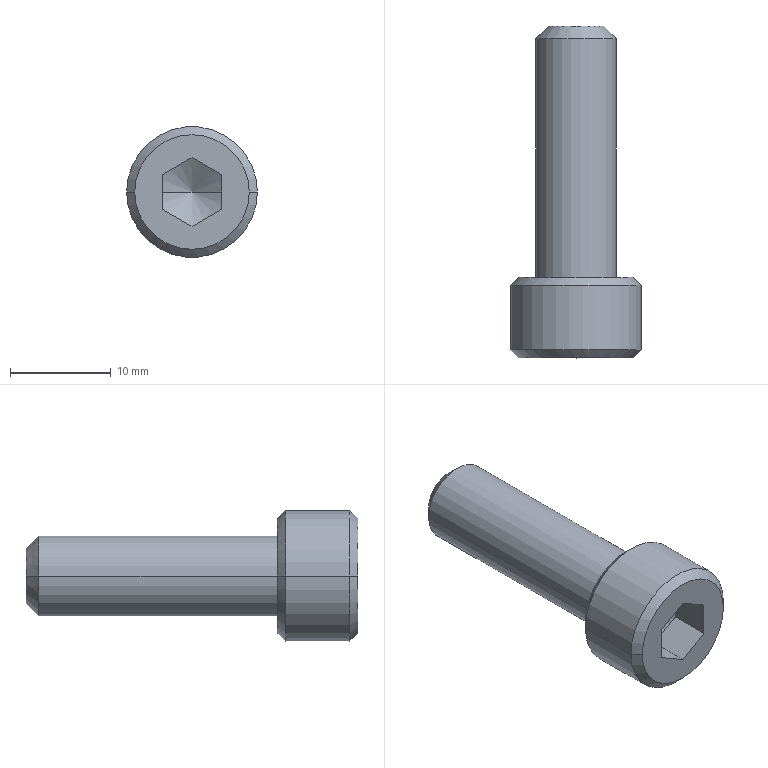Part | STEP file | BB62-M8-25L-1 | 1 solid | 27 faces | box 13 x 33 x 13 mm | volume 2129 mm3 | plane 15 | cone 8 | cylinder 4 | commonest cylinder face diameters 8 x2 13 x2
STEP:
#1=CARTESIAN_POINT('',(0.,-2.02,0.));
#2=VERTEX_POINT('',#1);
#3=CARTESIAN_POINT('',(3.43,-4.,0.));
#4=VERTEX_POINT('',#3);
#5=CARTESIAN_POINT('',(0.,-2.02,0.));
#6=DIRECTION('',(0.866,-0.5,0.));
#7=VECTOR('',#6,1000.);
#8=LINE('',#5,#7);
#9=EDGE_CURVE('',#2,#4,#8,.T.);
#10=ORIENTED_EDGE('',*,*,#9,.F.);
#11=CARTESIAN_POINT('',(-3.43,-4.,0.));
#12=VERTEX_POINT('',#11);
#13=CARTESIAN_POINT('',(0.,-2.02,0.));
#14=DIRECTION('',(-0.866,-0.5,0.));
#15=VECTOR('',#14,1000.);
#16=LINE('',#13,#15);
#17=EDGE_CURVE('',#2,#12,#16,.T.);
#18=ORIENTED_EDGE('',*,*,#17,.T.);
#19=CARTESIAN_POINT('',(-2.97,-4.,-1.715));
#20=VERTEX_POINT('',#19);
#21=CARTESIAN_POINT('',(0.,-4.,0.));
#22=DIRECTION('',(0.,-1.,0.));
#23=DIRECTION('',(-1.,0.,0.));
#24=AXIS2_PLACEMENT_3D('',#21,#22,#23);
#25=CIRCLE('',#24,3.43);
#26=EDGE_CURVE('',#12,#20,#25,.T.);
#27=ORIENTED_EDGE('',*,*,#26,.T.);
#28=CARTESIAN_POINT('',(0.,-4.,-3.43));
#29=VERTEX_POINT('',#28);
#30=CARTESIAN_POINT('',(0.,-4.,0.));
#31=DIRECTION('',(0.,-1.,0.));
#32=DIRECTION('',(-1.,0.,0.));
#33=AXIS2_PLACEMENT_3D('',#30,#31,#32);
#34=CIRCLE('',#33,3.43);
#35=EDGE_CURVE('',#20,#29,#34,.T.);
#36=ORIENTED_EDGE('',*,*,#35,.T.);
#37=CARTESIAN_POINT('',(2.97,-4.,-1.715));
#38=VERTEX_POINT('',#37);
#39=CARTESIAN_POINT('',(0.,-4.,0.));
#40=DIRECTION('',(0.,-1.,0.));
#41=DIRECTION('',(-1.,0.,0.));
#42=AXIS2_PLACEMENT_3D('',#39,#40,#41);
#43=CIRCLE('',#42,3.43);
#44=EDGE_CURVE('',#29,#38,#43,.T.);
#45=ORIENTED_EDGE('',*,*,#44,.T.);
#46=CARTESIAN_POINT('',(0.,-4.,0.));
#47=DIRECTION('',(0.,-1.,0.));
#48=DIRECTION('',(-1.,0.,0.));
#49=AXIS2_PLACEMENT_3D('',#46,#47,#48);
#50=CIRCLE('',#49,3.43);
#51=EDGE_CURVE('',#38,#4,#50,.T.);
#52=ORIENTED_EDGE('',*,*,#51,.T.);
#53=EDGE_LOOP('',(#10,#18,#27,#36,#45,#52));
#54=FACE_OUTER_BOUND('',#53,.T.);
#55=CARTESIAN_POINT('',(0.,-1002.02,0.));
#56=DIRECTION('',(0.,-1.,0.));
#57=DIRECTION('',(1.,0.,0.));
#58=AXIS2_PLACEMENT_3D('',#55,#56,#57);
#59=CONICAL_SURFACE('',#58,1732.051,1.047);
#60=ADVANCED_FACE('',(#54),#59,.F.);
#61=CARTESIAN_POINT('',(-2.75,25.,0.));
#62=VERTEX_POINT('',#61);
#63=CARTESIAN_POINT('',(2.75,25.,0.));
#64=VERTEX_POINT('',#63);
#65=CARTESIAN_POINT('',(0.,25.,0.));
#66=DIRECTION('',(0.,1.,0.));
#67=DIRECTION('',(1.,0.,0.));
#68=AXIS2_PLACEMENT_3D('',#65,#66,#67);
#69=CIRCLE('',#68,2.75);
#70=EDGE_CURVE('',#62,#64,#69,.T.);
#71=ORIENTED_EDGE('',*,*,#70,.F.);
#72=CARTESIAN_POINT('',(-4.,23.75,0.));
#73=VERTEX_POINT('',#72);
#74=CARTESIAN_POINT('',(-2.75,25.,0.));
#75=DIRECTION('',(-0.7071,-0.7071,0.));
#76=VECTOR('',#75,1000.);
#77=LINE('',#74,#76);
#78=EDGE_CURVE('',#62,#73,#77,.T.);
#79=ORIENTED_EDGE('',*,*,#78,.T.);
#80=CARTESIAN_POINT('',(4.,23.75,0.));
#81=VERTEX_POINT('',#80);
#82=CARTESIAN_POINT('',(0.,23.75,0.));
#83=DIRECTION('',(0.,-1.,0.));
#84=DIRECTION('',(-1.,0.,0.));
#85=AXIS2_PLACEMENT_3D('',#82,#83,#84);
#86=CIRCLE('',#85,4.);
#87=EDGE_CURVE('',#81,#73,#86,.T.);
#88=ORIENTED_EDGE('',*,*,#87,.F.);
#89=CARTESIAN_POINT('',(2.75,25.,0.));
#90=DIRECTION('',(0.7071,-0.7071,0.));
#91=VECTOR('',#90,1000.);
#92=LINE('',#89,#91);
#93=EDGE_CURVE('',#64,#81,#92,.T.);
#94=ORIENTED_EDGE('',*,*,#93,.F.);
#95=EDGE_LOOP('',(#71,#79,#88,#94));
#96=FACE_OUTER_BOUND('',#95,.T.);
#97=CARTESIAN_POINT('',(0.,25.,0.));
#98=DIRECTION('',(0.,-1.,0.));
#99=DIRECTION('',(1.,0.,0.));
#100=AXIS2_PLACEMENT_3D('',#97,#98,#99);
#101=CONICAL_SURFACE('',#100,2.75,0.7854);
#102=ADVANCED_FACE('',(#96),#101,.T.);
#103=ORIENTED_EDGE('',*,*,#87,.T.);
#104=CARTESIAN_POINT('',(-4.,0.,0.));
#105=VERTEX_POINT('',#104);
#106=CARTESIAN_POINT('',(-4.,23.75,0.));
#107=DIRECTION('',(0.,-1.,0.));
#108=VECTOR('',#107,1000.);
#109=LINE('',#106,#108);
#110=EDGE_CURVE('',#73,#105,#109,.T.);
#111=ORIENTED_EDGE('',*,*,#110,.T.);
#112=CARTESIAN_POINT('',(4.,0.,0.));
#113=VERTEX_POINT('',#112);
#114=CARTESIAN_POINT('',(0.,0.,0.));
#115=DIRECTION('',(0.,-1.,0.));
#116=DIRECTION('',(-1.,0.,0.));
#117=AXIS2_PLACEMENT_3D('',#114,#115,#116);
#118=CIRCLE('',#117,4.);
#119=EDGE_CURVE('',#113,#105,#118,.T.);
#120=ORIENTED_EDGE('',*,*,#119,.F.);
#121=CARTESIAN_POINT('',(4.,23.75,0.));
#122=DIRECTION('',(0.,-1.,0.));
#123=VECTOR('',#122,1000.);
#124=LINE('',#121,#123);
#125=EDGE_CURVE('',#81,#113,#124,.T.);
#126=ORIENTED_EDGE('',*,*,#125,.F.);
#127=EDGE_LOOP('',(#103,#111,#120,#126));
#128=FACE_OUTER_BOUND('',#127,.T.);
#129=CARTESIAN_POINT('',(0.,23.75,0.));
#130=DIRECTION('',(0.,-1.,0.));
#131=DIRECTION('',(1.,0.,0.));
#132=AXIS2_PLACEMENT_3D('',#129,#130,#131);
#133=CYLINDRICAL_SURFACE('',#132,4.);
#134=ADVANCED_FACE('',(#128),#133,.T.);
#135=CARTESIAN_POINT('',(5.7,-8.,0.));
#136=VERTEX_POINT('',#135);
#137=CARTESIAN_POINT('',(-5.7,-8.,0.));
#138=VERTEX_POINT('',#137);
#139=CARTESIAN_POINT('',(0.,-8.,0.));
#140=DIRECTION('',(0.,-1.,0.));
#141=DIRECTION('',(-1.,0.,0.));
#142=AXIS2_PLACEMENT_3D('',#139,#140,#141);
#143=CIRCLE('',#142,5.7);
#144=EDGE_CURVE('',#136,#138,#143,.T.);
#145=ORIENTED_EDGE('',*,*,#144,.F.);
#146=CARTESIAN_POINT('',(6.5,-7.2,0.));
#147=VERTEX_POINT('',#146);
#148=CARTESIAN_POINT('',(6.5,-7.2,0.));
#149=DIRECTION('',(0.7071,0.7071,0.));
#150=VECTOR('',#149,1000.);
#151=LINE('',#148,#150);
#152=EDGE_CURVE('',#136,#147,#151,.T.);
#153=ORIENTED_EDGE('',*,*,#152,.T.);
#154=CARTESIAN_POINT('',(-6.5,-7.2,0.));
#155=VERTEX_POINT('',#154);
#156=CARTESIAN_POINT('',(0.,-7.2,0.));
#157=DIRECTION('',(0.,-1.,0.));
#158=DIRECTION('',(-1.,0.,0.));
#159=AXIS2_PLACEMENT_3D('',#156,#157,#158);
#160=CIRCLE('',#159,6.5);
#161=EDGE_CURVE('',#147,#155,#160,.T.);
#162=ORIENTED_EDGE('',*,*,#161,.T.);
#163=CARTESIAN_POINT('',(-6.5,-7.2,0.));
#164=DIRECTION('',(-0.7071,0.7071,0.));
#165=VECTOR('',#164,1000.);
#166=LINE('',#163,#165);
#167=EDGE_CURVE('',#138,#155,#166,.T.);
#168=ORIENTED_EDGE('',*,*,#167,.F.);
#169=EDGE_LOOP('',(#145,#153,#162,#168));
#170=FACE_OUTER_BOUND('',#169,.T.);
#171=CARTESIAN_POINT('',(0.,-7.2,0.));
#172=DIRECTION('',(0.,1.,0.));
#173=DIRECTION('',(-1.,0.,0.));
#174=AXIS2_PLACEMENT_3D('',#171,#172,#173);
#175=CONICAL_SURFACE('',#174,6.5,0.7854);
#176=ADVANCED_FACE('',(#170),#175,.T.);
#177=ORIENTED_EDGE('',*,*,#161,.F.);
#178=CARTESIAN_POINT('',(6.5,-0.8,0.));
#179=VERTEX_POINT('',#178);
#180=CARTESIAN_POINT('',(6.5,-1.62,0.));
#181=DIRECTION('',(0.,1.,0.));
#182=VECTOR('',#181,1000.);
#183=LINE('',#180,#182);
#184=EDGE_CURVE('',#147,#179,#183,.T.);
#185=ORIENTED_EDGE('',*,*,#184,.T.);
#186=CARTESIAN_POINT('',(-6.5,-0.8,0.));
#187=VERTEX_POINT('',#186);
#188=CARTESIAN_POINT('',(0.,-0.8,0.));
#189=DIRECTION('',(0.,-1.,0.));
#190=DIRECTION('',(-1.,0.,0.));
#191=AXIS2_PLACEMENT_3D('',#188,#189,#190);
#192=CIRCLE('',#191,6.5);
#193=EDGE_CURVE('',#179,#187,#192,.T.);
#194=ORIENTED_EDGE('',*,*,#193,.T.);
#195=CARTESIAN_POINT('',(-6.5,-1.62,0.));
#196=DIRECTION('',(0.,1.,0.));
#197=VECTOR('',#196,1000.);
#198=LINE('',#195,#197);
#199=EDGE_CURVE('',#155,#187,#198,.T.);
#200=ORIENTED_EDGE('',*,*,#199,.F.);
#201=EDGE_LOOP('',(#177,#185,#194,#200));
#202=FACE_OUTER_BOUND('',#201,.T.);
#203=CARTESIAN_POINT('',(0.,-1.62,0.));
#204=DIRECTION('',(0.,1.,0.));
#205=DIRECTION('',(-1.,0.,0.));
#206=AXIS2_PLACEMENT_3D('',#203,#204,#205);
#207=CYLINDRICAL_SURFACE('',#206,6.5);
#208=ADVANCED_FACE('',(#202),#207,.T.);
#209=CARTESIAN_POINT('',(5.7,0.,0.));
#210=VERTEX_POINT('',#209);
#211=CARTESIAN_POINT('',(-5.7,0.,0.));
#212=VERTEX_POINT('',#211);
#213=CARTESIAN_POINT('',(0.,0.,0.));
#214=DIRECTION('',(0.,-1.,0.));
#215=DIRECTION('',(-1.,0.,0.));
#216=AXIS2_PLACEMENT_3D('',#213,#214,#215);
#217=CIRCLE('',#216,5.7);
#218=EDGE_CURVE('',#210,#212,#217,.T.);
#219=ORIENTED_EDGE('',*,*,#218,.T.);
#220=CARTESIAN_POINT('',(-5.7,0.,0.));
#221=DIRECTION('',(-0.7071,-0.7071,0.));
#222=VECTOR('',#221,1000.);
#223=LINE('',#220,#222);
#224=EDGE_CURVE('',#212,#187,#223,.T.);
#225=ORIENTED_EDGE('',*,*,#224,.T.);
#226=ORIENTED_EDGE('',*,*,#193,.F.);
#227=CARTESIAN_POINT('',(5.7,0.,0.));
#228=DIRECTION('',(0.7071,-0.7071,0.));
#229=VECTOR('',#228,1000.);
#230=LINE('',#227,#229);
#231=EDGE_CURVE('',#210,#179,#230,.T.);
#232=ORIENTED_EDGE('',*,*,#231,.F.);
#233=EDGE_LOOP('',(#219,#225,#226,#232));
#234=FACE_OUTER_BOUND('',#233,.T.);
#235=CARTESIAN_POINT('',(0.,0.,0.));
#236=DIRECTION('',(0.,-1.,0.));
#237=DIRECTION('',(1.,0.,0.));
#238=AXIS2_PLACEMENT_3D('',#235,#236,#237);
#239=CONICAL_SURFACE('',#238,5.7,0.7854);
#240=ADVANCED_FACE('',(#234),#239,.T.);
#241=CARTESIAN_POINT('',(0.,-8.,0.));
#242=DIRECTION('',(0.,-1.,0.));
#243=DIRECTION('',(-1.,0.,0.));
#244=AXIS2_PLACEMENT_3D('',#241,#242,#243);
#245=CIRCLE('',#244,5.7);
#246=EDGE_CURVE('',#138,#136,#245,.T.);
#247=ORIENTED_EDGE('',*,*,#246,.T.);
#248=ORIENTED_EDGE('',*,*,#144,.T.);
#249=EDGE_LOOP('',(#247,#248));
#250=FACE_OUTER_BOUND('',#249,.T.);
#251=CARTESIAN_POINT('',(0.,-8.,-3.43));
#252=VERTEX_POINT('',#251);
#253=CARTESIAN_POINT('',(-2.97,-8.,-1.715));
#254=VERTEX_POINT('',#253);
#255=CARTESIAN_POINT('',(0.,-8.,-3.43));
#256=DIRECTION('',(-0.866,0.,0.5));
#257=VECTOR('',#256,1000.);
#258=LINE('',#255,#257);
#259=EDGE_CURVE('',#252,#254,#258,.T.);
#260=ORIENTED_EDGE('',*,*,#259,.T.);
#261=CARTESIAN_POINT('',(-2.97,-8.,1.715));
#262=VERTEX_POINT('',#261);
#263=CARTESIAN_POINT('',(-2.97,-8.,-1.715));
#264=DIRECTION('',(0.,0.,1.));
#265=VECTOR('',#264,1000.);
#266=LINE('',#263,#265);
#267=EDGE_CURVE('',#254,#262,#266,.T.);
#268=ORIENTED_EDGE('',*,*,#267,.T.);
#269=CARTESIAN_POINT('',(0.,-8.,3.43));
#270=VERTEX_POINT('',#269);
#271=CARTESIAN_POINT('',(-2.97,-8.,1.715));
#272=DIRECTION('',(0.866,0.,0.5));
#273=VECTOR('',#272,1000.);
#274=LINE('',#271,#273);
#275=EDGE_CURVE('',#262,#270,#274,.T.);
#276=ORIENTED_EDGE('',*,*,#275,.T.);
#277=CARTESIAN_POINT('',(2.97,-8.,1.715));
#278=VERTEX_POINT('',#277);
#279=CARTESIAN_POINT('',(0.,-8.,3.43));
#280=DIRECTION('',(0.866,0.,-0.5));
#281=VECTOR('',#280,1000.);
#282=LINE('',#279,#281);
#283=EDGE_CURVE('',#270,#278,#282,.T.);
#284=ORIENTED_EDGE('',*,*,#283,.T.);
#285=CARTESIAN_POINT('',(2.97,-8.,-1.715));
#286=VERTEX_POINT('',#285);
#287=CARTESIAN_POINT('',(2.97,-8.,1.715));
#288=DIRECTION('',(0.,0.,-1.));
#289=VECTOR('',#288,1000.);
#290=LINE('',#287,#289);
#291=EDGE_CURVE('',#278,#286,#290,.T.);
#292=ORIENTED_EDGE('',*,*,#291,.T.);
#293=CARTESIAN_POINT('',(2.97,-8.,-1.715));
#294=DIRECTION('',(-0.866,0.,-0.5));
#295=VECTOR('',#294,1000.);
#296=LINE('',#293,#295);
#297=EDGE_CURVE('',#286,#252,#296,.T.);
#298=ORIENTED_EDGE('',*,*,#297,.T.);
#299=EDGE_LOOP('',(#260,#268,#276,#284,#292,#298));
#300=FACE_BOUND('',#299,.T.);
#301=CARTESIAN_POINT('',(5.7,-8.,0.));
#302=DIRECTION('',(0.,-1.,0.));
#303=DIRECTION('',(1.,0.,0.));
#304=AXIS2_PLACEMENT_3D('',#301,#302,#303);
#305=PLANE('',#304);
#306=ADVANCED_FACE('',(#250,#300),#305,.T.);
#307=ORIENTED_EDGE('',*,*,#119,.T.);
#308=CARTESIAN_POINT('',(0.,0.,0.));
#309=DIRECTION('',(0.,-1.,0.));
#310=DIRECTION('',(-1.,0.,0.));
#311=AXIS2_PLACEMENT_3D('',#308,#309,#310);
#312=CIRCLE('',#311,4.);
#313=EDGE_CURVE('',#105,#113,#312,.T.);
#314=ORIENTED_EDGE('',*,*,#313,.T.);
#315=EDGE_LOOP('',(#307,#314));
#316=FACE_BOUND('',#315,.T.);
#317=ORIENTED_EDGE('',*,*,#218,.F.);
#318=CARTESIAN_POINT('',(0.,0.,0.));
#319=DIRECTION('',(0.,-1.,0.));
#320=DIRECTION('',(-1.,0.,0.));
#321=AXIS2_PLACEMENT_3D('',#318,#319,#320);
#322=CIRCLE('',#321,5.7);
#323=EDGE_CURVE('',#212,#210,#322,.T.);
#324=ORIENTED_EDGE('',*,*,#323,.F.);
#325=EDGE_LOOP('',(#317,#324));
#326=FACE_OUTER_BOUND('',#325,.T.);
#327=CARTESIAN_POINT('',(0.,0.,0.));
#328=DIRECTION('',(0.,1.,0.));
#329=DIRECTION('',(-1.,0.,0.));
#330=AXIS2_PLACEMENT_3D('',#327,#328,#329);
#331=PLANE('',#330);
#332=ADVANCED_FACE('',(#316,#326),#331,.T.);
#333=ORIENTED_EDGE('',*,*,#224,.F.);
#334=ORIENTED_EDGE('',*,*,#323,.T.);
#335=ORIENTED_EDGE('',*,*,#231,.T.);
#336=CARTESIAN_POINT('',(0.,-0.8,0.));
#337=DIRECTION('',(0.,-1.,0.));
#338=DIRECTION('',(-1.,0.,0.));
#339=AXIS2_PLACEMENT_3D('',#336,#337,#338);
#340=CIRCLE('',#339,6.5);
#341=EDGE_CURVE('',#187,#179,#340,.T.);
#342=ORIENTED_EDGE('',*,*,#341,.F.);
#343=EDGE_LOOP('',(#333,#334,#335,#342));
#344=FACE_OUTER_BOUND('',#343,.T.);
#345=CARTESIAN_POINT('',(0.,0.,0.));
#346=DIRECTION('',(0.,-1.,0.));
#347=DIRECTION('',(1.,0.,0.));
#348=AXIS2_PLACEMENT_3D('',#345,#346,#347);
#349=CONICAL_SURFACE('',#348,5.7,0.7854);
#350=ADVANCED_FACE('',(#344),#349,.T.);
#351=ORIENTED_EDGE('',*,*,#184,.F.);
#352=CARTESIAN_POINT('',(0.,-7.2,0.));
#353=DIRECTION('',(0.,-1.,0.));
#354=DIRECTION('',(-1.,0.,0.));
#355=AXIS2_PLACEMENT_3D('',#352,#353,#354);
#356=CIRCLE('',#355,6.5);
#357=EDGE_CURVE('',#155,#147,#356,.T.);
#358=ORIENTED_EDGE('',*,*,#357,.F.);
#359=ORIENTED_EDGE('',*,*,#199,.T.);
#360=ORIENTED_EDGE('',*,*,#341,.T.);
#361=EDGE_LOOP('',(#351,#358,#359,#360));
#362=FACE_OUTER_BOUND('',#361,.T.);
#363=CARTESIAN_POINT('',(0.,-1.62,0.));
#364=DIRECTION('',(0.,1.,0.));
#365=DIRECTION('',(-1.,0.,0.));
#366=AXIS2_PLACEMENT_3D('',#363,#364,#365);
#367=CYLINDRICAL_SURFACE('',#366,6.5);
#368=ADVANCED_FACE('',(#362),#367,.T.);
#369=ORIENTED_EDGE('',*,*,#152,.F.);
#370=ORIENTED_EDGE('',*,*,#246,.F.);
#371=ORIENTED_EDGE('',*,*,#167,.T.);
#372=ORIENTED_EDGE('',*,*,#357,.T.);
#373=EDGE_LOOP('',(#369,#370,#371,#372));
#374=FACE_OUTER_BOUND('',#373,.T.);
#375=CARTESIAN_POINT('',(0.,-7.2,0.));
#376=DIRECTION('',(0.,1.,0.));
#377=DIRECTION('',(-1.,0.,0.));
#378=AXIS2_PLACEMENT_3D('',#375,#376,#377);
#379=CONICAL_SURFACE('',#378,6.5,0.7854);
#380=ADVANCED_FACE('',(#374),#379,.T.);
#381=ORIENTED_EDGE('',*,*,#110,.F.);
#382=CARTESIAN_POINT('',(0.,23.75,0.));
#383=DIRECTION('',(0.,-1.,0.));
#384=DIRECTION('',(-1.,0.,0.));
#385=AXIS2_PLACEMENT_3D('',#382,#383,#384);
#386=CIRCLE('',#385,4.);
#387=EDGE_CURVE('',#73,#81,#386,.T.);
#388=ORIENTED_EDGE('',*,*,#387,.T.);
#389=ORIENTED_EDGE('',*,*,#125,.T.);
#390=ORIENTED_EDGE('',*,*,#313,.F.);
#391=EDGE_LOOP('',(#381,#388,#389,#390));
#392=FACE_OUTER_BOUND('',#391,.T.);
#393=CARTESIAN_POINT('',(0.,23.75,0.));
#394=DIRECTION('',(0.,-1.,0.));
#395=DIRECTION('',(1.,0.,0.));
#396=AXIS2_PLACEMENT_3D('',#393,#394,#395);
#397=CYLINDRICAL_SURFACE('',#396,4.);
#398=ADVANCED_FACE('',(#392),#397,.T.);
#399=CARTESIAN_POINT('',(0.,25.,0.));
#400=DIRECTION('',(0.,1.,0.));
#401=DIRECTION('',(1.,0.,0.));
#402=AXIS2_PLACEMENT_3D('',#399,#400,#401);
#403=CIRCLE('',#402,2.75);
#404=EDGE_CURVE('',#64,#62,#403,.T.);
#405=ORIENTED_EDGE('',*,*,#404,.T.);
#406=ORIENTED_EDGE('',*,*,#70,.T.);
#407=EDGE_LOOP('',(#405,#406));
#408=FACE_OUTER_BOUND('',#407,.T.);
#409=CARTESIAN_POINT('',(0.,25.,0.));
#410=DIRECTION('',(0.,1.,0.));
#411=DIRECTION('',(-1.,0.,0.));
#412=AXIS2_PLACEMENT_3D('',#409,#410,#411);
#413=PLANE('',#412);
#414=ADVANCED_FACE('',(#408),#413,.T.);
#415=ORIENTED_EDGE('',*,*,#78,.F.);
#416=ORIENTED_EDGE('',*,*,#404,.F.);
#417=ORIENTED_EDGE('',*,*,#93,.T.);
#418=ORIENTED_EDGE('',*,*,#387,.F.);
#419=EDGE_LOOP('',(#415,#416,#417,#418));
#420=FACE_OUTER_BOUND('',#419,.T.);
#421=CARTESIAN_POINT('',(0.,25.,0.));
#422=DIRECTION('',(0.,-1.,0.));
#423=DIRECTION('',(1.,0.,0.));
#424=AXIS2_PLACEMENT_3D('',#421,#422,#423);
#425=CONICAL_SURFACE('',#424,2.75,0.7854);
#426=ADVANCED_FACE('',(#420),#425,.T.);
#427=CARTESIAN_POINT('',(2.97,-4.,-1.715));
#428=DIRECTION('',(-0.866,0.,-0.5));
#429=VECTOR('',#428,1000.);
#430=LINE('',#427,#429);
#431=EDGE_CURVE('',#38,#29,#430,.T.);
#432=ORIENTED_EDGE('',*,*,#431,.T.);
#433=CARTESIAN_POINT('',(0.,-8.,-3.43));
#434=DIRECTION('',(0.,1.,0.));
#435=VECTOR('',#434,1000.);
#436=LINE('',#433,#435);
#437=EDGE_CURVE('',#252,#29,#436,.T.);
#438=ORIENTED_EDGE('',*,*,#437,.F.);
#439=ORIENTED_EDGE('',*,*,#297,.F.);
#440=CARTESIAN_POINT('',(2.97,-8.,-1.715));
#441=DIRECTION('',(0.,1.,0.));
#442=VECTOR('',#441,1000.);
#443=LINE('',#440,#442);
#444=EDGE_CURVE('',#286,#38,#443,.T.);
#445=ORIENTED_EDGE('',*,*,#444,.T.);
#446=EDGE_LOOP('',(#432,#438,#439,#445));
#447=FACE_OUTER_BOUND('',#446,.T.);
#448=CARTESIAN_POINT('',(2.97,-8.,-1.715));
#449=DIRECTION('',(-0.5,0.,0.866));
#450=DIRECTION('',(0.866,0.,0.5));
#451=AXIS2_PLACEMENT_3D('',#448,#449,#450);
#452=PLANE('',#451);
#453=ADVANCED_FACE('',(#447),#452,.T.);
#454=CARTESIAN_POINT('',(0.,-4.,-3.43));
#455=DIRECTION('',(-0.866,0.,0.5));
#456=VECTOR('',#455,1000.);
#457=LINE('',#454,#456);
#458=EDGE_CURVE('',#29,#20,#457,.T.);
#459=ORIENTED_EDGE('',*,*,#458,.T.);
#460=CARTESIAN_POINT('',(-2.97,-8.,-1.715));
#461=DIRECTION('',(0.,1.,0.));
#462=VECTOR('',#461,1000.);
#463=LINE('',#460,#462);
#464=EDGE_CURVE('',#254,#20,#463,.T.);
#465=ORIENTED_EDGE('',*,*,#464,.F.);
#466=ORIENTED_EDGE('',*,*,#259,.F.);
#467=ORIENTED_EDGE('',*,*,#437,.T.);
#468=EDGE_LOOP('',(#459,#465,#466,#467));
#469=FACE_OUTER_BOUND('',#468,.T.);
#470=CARTESIAN_POINT('',(0.,-8.,-3.43));
#471=DIRECTION('',(0.5,0.,0.866));
#472=DIRECTION('',(0.866,0.,-0.5));
#473=AXIS2_PLACEMENT_3D('',#470,#471,#472);
#474=PLANE('',#473);
#475=ADVANCED_FACE('',(#469),#474,.T.);
#476=CARTESIAN_POINT('',(-2.97,-4.,1.715));
#477=VERTEX_POINT('',#476);
#478=CARTESIAN_POINT('',(-2.97,-4.,-1.715));
#479=DIRECTION('',(0.,0.,1.));
#480=VECTOR('',#479,1000.);
#481=LINE('',#478,#480);
#482=EDGE_CURVE('',#20,#477,#481,.T.);
#483=ORIENTED_EDGE('',*,*,#482,.T.);
#484=CARTESIAN_POINT('',(-2.97,-8.,1.715));
#485=DIRECTION('',(0.,1.,0.));
#486=VECTOR('',#485,1000.);
#487=LINE('',#484,#486);
#488=EDGE_CURVE('',#262,#477,#487,.T.);
#489=ORIENTED_EDGE('',*,*,#488,.F.);
#490=ORIENTED_EDGE('',*,*,#267,.F.);
#491=ORIENTED_EDGE('',*,*,#464,.T.);
#492=EDGE_LOOP('',(#483,#489,#490,#491));
#493=FACE_OUTER_BOUND('',#492,.T.);
#494=CARTESIAN_POINT('',(-2.97,-8.,-1.715));
#495=DIRECTION('',(1.,0.,0.));
#496=DIRECTION('',(0.,0.,-1.));
#497=AXIS2_PLACEMENT_3D('',#494,#495,#496);
#498=PLANE('',#497);
#499=ADVANCED_FACE('',(#493),#498,.T.);
#500=CARTESIAN_POINT('',(0.,-4.,3.43));
#501=VERTEX_POINT('',#500);
#502=CARTESIAN_POINT('',(-2.97,-4.,1.715));
#503=DIRECTION('',(0.866,0.,0.5));
#504=VECTOR('',#503,1000.);
#505=LINE('',#502,#504);
#506=EDGE_CURVE('',#477,#501,#505,.T.);
#507=ORIENTED_EDGE('',*,*,#506,.T.);
#508=CARTESIAN_POINT('',(0.,-8.,3.43));
#509=DIRECTION('',(0.,1.,0.));
#510=VECTOR('',#509,1000.);
#511=LINE('',#508,#510);
#512=EDGE_CURVE('',#270,#501,#511,.T.);
#513=ORIENTED_EDGE('',*,*,#512,.F.);
#514=ORIENTED_EDGE('',*,*,#275,.F.);
#515=ORIENTED_EDGE('',*,*,#488,.T.);
#516=EDGE_LOOP('',(#507,#513,#514,#515));
#517=FACE_OUTER_BOUND('',#516,.T.);
#518=CARTESIAN_POINT('',(-2.97,-8.,1.715));
#519=DIRECTION('',(0.5,0.,-0.866));
#520=DIRECTION('',(-0.866,0.,-0.5));
#521=AXIS2_PLACEMENT_3D('',#518,#519,#520);
#522=PLANE('',#521);
#523=ADVANCED_FACE('',(#517),#522,.T.);
#524=CARTESIAN_POINT('',(2.97,-4.,1.715));
#525=VERTEX_POINT('',#524);
#526=CARTESIAN_POINT('',(0.,-4.,3.43));
#527=DIRECTION('',(0.866,0.,-0.5));
#528=VECTOR('',#527,1000.);
#529=LINE('',#526,#528);
#530=EDGE_CURVE('',#501,#525,#529,.T.);
#531=ORIENTED_EDGE('',*,*,#530,.T.);
#532=CARTESIAN_POINT('',(2.97,-8.,1.715));
#533=DIRECTION('',(0.,1.,0.));
#534=VECTOR('',#533,1000.);
#535=LINE('',#532,#534);
#536=EDGE_CURVE('',#278,#525,#535,.T.);
#537=ORIENTED_EDGE('',*,*,#536,.F.);
#538=ORIENTED_EDGE('',*,*,#283,.F.);
#539=ORIENTED_EDGE('',*,*,#512,.T.);
#540=EDGE_LOOP('',(#531,#537,#538,#539));
#541=FACE_OUTER_BOUND('',#540,.T.);
#542=CARTESIAN_POINT('',(0.,-8.,3.43));
#543=DIRECTION('',(-0.5,0.,-0.866));
#544=DIRECTION('',(-0.866,0.,0.5));
#545=AXIS2_PLACEMENT_3D('',#542,#543,#544);
#546=PLANE('',#545);
#547=ADVANCED_FACE('',(#541),#546,.T.);
#548=CARTESIAN_POINT('',(2.97,-4.,1.715));
#549=DIRECTION('',(0.,0.,-1.));
#550=VECTOR('',#549,1000.);
#551=LINE('',#548,#550);
#552=EDGE_CURVE('',#525,#38,#551,.T.);
#553=ORIENTED_EDGE('',*,*,#552,.T.);
#554=ORIENTED_EDGE('',*,*,#444,.F.);
#555=ORIENTED_EDGE('',*,*,#291,.F.);
#556=ORIENTED_EDGE('',*,*,#536,.T.);
#557=EDGE_LOOP('',(#553,#554,#555,#556));
#558=FACE_OUTER_BOUND('',#557,.T.);
#559=CARTESIAN_POINT('',(2.97,-8.,1.715));
#560=DIRECTION('',(-1.,0.,0.));
#561=DIRECTION('',(0.,0.,1.));
#562=AXIS2_PLACEMENT_3D('',#559,#560,#561);
#563=PLANE('',#562);
#564=ADVANCED_FACE('',(#558),#563,.T.);
#565=ORIENTED_EDGE('',*,*,#431,.F.);
#566=ORIENTED_EDGE('',*,*,#44,.F.);
#567=EDGE_LOOP('',(#565,#566));
#568=FACE_OUTER_BOUND('',#567,.T.);
#569=CARTESIAN_POINT('',(0.,-4.,0.));
#570=DIRECTION('',(0.,-1.,0.));
#571=DIRECTION('',(1.,0.,0.));
#572=AXIS2_PLACEMENT_3D('',#569,#570,#571);
#573=PLANE('',#572);
#574=ADVANCED_FACE('',(#568),#573,.F.);
#575=ORIENTED_EDGE('',*,*,#552,.F.);
#576=CARTESIAN_POINT('',(0.,-4.,0.));
#577=DIRECTION('',(0.,-1.,0.));
#578=DIRECTION('',(-1.,0.,0.));
#579=AXIS2_PLACEMENT_3D('',#576,#577,#578);
#580=CIRCLE('',#579,3.43);
#581=EDGE_CURVE('',#4,#525,#580,.T.);
#582=ORIENTED_EDGE('',*,*,#581,.F.);
#583=ORIENTED_EDGE('',*,*,#51,.F.);
#584=EDGE_LOOP('',(#575,#582,#583));
#585=FACE_OUTER_BOUND('',#584,.T.);
#586=CARTESIAN_POINT('',(0.,-4.,0.));
#587=DIRECTION('',(0.,-1.,0.));
#588=DIRECTION('',(1.,0.,0.));
#589=AXIS2_PLACEMENT_3D('',#586,#587,#588);
#590=PLANE('',#589);
#591=ADVANCED_FACE('',(#585),#590,.F.);
#592=ORIENTED_EDGE('',*,*,#530,.F.);
#593=CARTESIAN_POINT('',(0.,-4.,0.));
#594=DIRECTION('',(0.,-1.,0.));
#595=DIRECTION('',(-1.,0.,0.));
#596=AXIS2_PLACEMENT_3D('',#593,#594,#595);
#597=CIRCLE('',#596,3.43);
#598=EDGE_CURVE('',#525,#501,#597,.T.);
#599=ORIENTED_EDGE('',*,*,#598,.F.);
#600=EDGE_LOOP('',(#592,#599));
#601=FACE_OUTER_BOUND('',#600,.T.);
#602=CARTESIAN_POINT('',(0.,-4.,0.));
#603=DIRECTION('',(0.,-1.,0.));
#604=DIRECTION('',(1.,0.,0.));
#605=AXIS2_PLACEMENT_3D('',#602,#603,#604);
#606=PLANE('',#605);
#607=ADVANCED_FACE('',(#601),#606,.F.);
#608=ORIENTED_EDGE('',*,*,#506,.F.);
#609=CARTESIAN_POINT('',(0.,-4.,0.));
#610=DIRECTION('',(0.,-1.,0.));
#611=DIRECTION('',(-1.,0.,0.));
#612=AXIS2_PLACEMENT_3D('',#609,#610,#611);
#613=CIRCLE('',#612,3.43);
#614=EDGE_CURVE('',#501,#477,#613,.T.);
#615=ORIENTED_EDGE('',*,*,#614,.F.);
#616=EDGE_LOOP('',(#608,#615));
#617=FACE_OUTER_BOUND('',#616,.T.);
#618=CARTESIAN_POINT('',(0.,-4.,0.));
#619=DIRECTION('',(0.,-1.,0.));
#620=DIRECTION('',(1.,0.,0.));
#621=AXIS2_PLACEMENT_3D('',#618,#619,#620);
#622=PLANE('',#621);
#623=ADVANCED_FACE('',(#617),#622,.F.);
#624=ORIENTED_EDGE('',*,*,#482,.F.);
#625=ORIENTED_EDGE('',*,*,#26,.F.);
#626=CARTESIAN_POINT('',(0.,-4.,0.));
#627=DIRECTION('',(0.,-1.,0.));
#628=DIRECTION('',(-1.,0.,0.));
#629=AXIS2_PLACEMENT_3D('',#626,#627,#628);
#630=CIRCLE('',#629,3.43);
#631=EDGE_CURVE('',#477,#12,#630,.T.);
#632=ORIENTED_EDGE('',*,*,#631,.F.);
#633=EDGE_LOOP('',(#624,#625,#632));
#634=FACE_OUTER_BOUND('',#633,.T.);
#635=CARTESIAN_POINT('',(0.,-4.,0.));
#636=DIRECTION('',(0.,-1.,0.));
#637=DIRECTION('',(1.,0.,0.));
#638=AXIS2_PLACEMENT_3D('',#635,#636,#637);
#639=PLANE('',#638);
#640=ADVANCED_FACE('',(#634),#639,.F.);
#641=ORIENTED_EDGE('',*,*,#458,.F.);
#642=ORIENTED_EDGE('',*,*,#35,.F.);
#643=EDGE_LOOP('',(#641,#642));
#644=FACE_OUTER_BOUND('',#643,.T.);
#645=CARTESIAN_POINT('',(0.,-4.,0.));
#646=DIRECTION('',(0.,-1.,0.));
#647=DIRECTION('',(1.,0.,0.));
#648=AXIS2_PLACEMENT_3D('',#645,#646,#647);
#649=PLANE('',#648);
#650=ADVANCED_FACE('',(#644),#649,.F.);
#651=ORIENTED_EDGE('',*,*,#17,.F.);
#652=ORIENTED_EDGE('',*,*,#9,.T.);
#653=ORIENTED_EDGE('',*,*,#581,.T.);
#654=ORIENTED_EDGE('',*,*,#598,.T.);
#655=ORIENTED_EDGE('',*,*,#614,.T.);
#656=ORIENTED_EDGE('',*,*,#631,.T.);
#657=EDGE_LOOP('',(#651,#652,#653,#654,#655,#656));
#658=FACE_OUTER_BOUND('',#657,.T.);
#659=CARTESIAN_POINT('',(0.,-1002.02,0.));
#660=DIRECTION('',(0.,-1.,0.));
#661=DIRECTION('',(1.,0.,0.));
#662=AXIS2_PLACEMENT_3D('',#659,#660,#661);
#663=CONICAL_SURFACE('',#662,1732.051,1.047);
#664=ADVANCED_FACE('',(#658),#663,.F.);
#665=CLOSED_SHELL('',(#60,#102,#134,#176,#208,#240,#306,#332,#350,#368,#380,#398,#414,#426,#453,#475,#499,#523,#547,#564,#574,#591,#607,#623,#640,#650,#664));
#666=MANIFOLD_SOLID_BREP('',#665);
#667=CARTESIAN_POINT('',(0.,0.,0.));
#668=DIRECTION('',(0.,0.,1.));
#669=DIRECTION('',(1.,0.,0.));
#670=AXIS2_PLACEMENT_3D('',#667,#668,#669);
#671=(LENGTH_UNIT()NAMED_UNIT(*)SI_UNIT(.MILLI.,.METRE.));
#672=UNCERTAINTY_MEASURE_WITH_UNIT(LENGTH_MEASURE(0.00001),#671,'','');
#673=(NAMED_UNIT(*)PLANE_ANGLE_UNIT()SI_UNIT($,.RADIAN.));
#674=(NAMED_UNIT(*)SI_UNIT($,.STERADIAN.)SOLID_ANGLE_UNIT());
#675=(GEOMETRIC_REPRESENTATION_CONTEXT(3)GLOBAL_UNCERTAINTY_ASSIGNED_CONTEXT((#672))GLOBAL_UNIT_ASSIGNED_CONTEXT((#671,#673,#674))REPRESENTATION_CONTEXT('',''));
#676=ADVANCED_BREP_SHAPE_REPRESENTATION('',(#666,#670),#675);